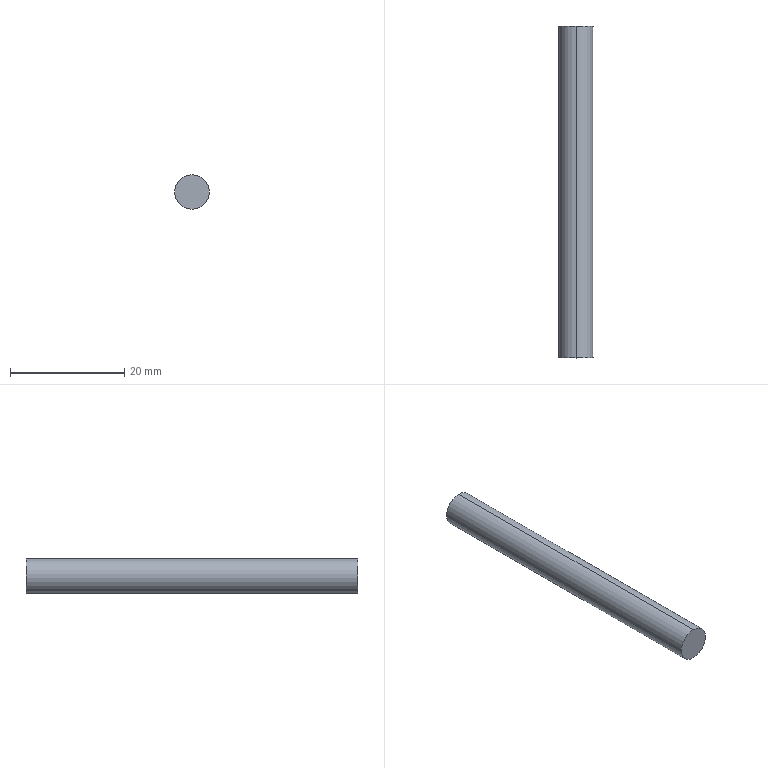Part | SolidWorks | features Extrusion 1 | 1 solid | 4 faces | box 6 x 58 x 6 mm | volume 1640 mm3 | cylinder 2 | plane 2 | commonest cylinder face diameters 6 x2
STEP:
#1=CARTESIAN_POINT('',(0.,58.,3.));
#2=VERTEX_POINT('',#1);
#3=CARTESIAN_POINT('',(0.,58.,-3.));
#4=VERTEX_POINT('',#3);
#5=CARTESIAN_POINT('',(0.,58.,0.));
#6=DIRECTION('',(0.,1.,0.));
#7=DIRECTION('',(0.,0.,1.));
#8=AXIS2_PLACEMENT_3D('',#5,#6,#7);
#9=CIRCLE('',#8,3.);
#10=EDGE_CURVE('',#2,#4,#9,.T.);
#11=ORIENTED_EDGE('',*,*,#10,.F.);
#12=CARTESIAN_POINT('',(0.,0.,3.));
#13=VERTEX_POINT('',#12);
#14=CARTESIAN_POINT('',(0.,58.,3.));
#15=DIRECTION('',(0.,-1.,0.));
#16=VECTOR('',#15,1000.);
#17=LINE('',#14,#16);
#18=EDGE_CURVE('',#2,#13,#17,.T.);
#19=ORIENTED_EDGE('',*,*,#18,.T.);
#20=CARTESIAN_POINT('',(0.,0.,-3.));
#21=VERTEX_POINT('',#20);
#22=CARTESIAN_POINT('',(0.,0.,0.));
#23=DIRECTION('',(0.,1.,0.));
#24=DIRECTION('',(0.,0.,1.));
#25=AXIS2_PLACEMENT_3D('',#22,#23,#24);
#26=CIRCLE('',#25,3.);
#27=EDGE_CURVE('',#13,#21,#26,.T.);
#28=ORIENTED_EDGE('',*,*,#27,.T.);
#29=CARTESIAN_POINT('',(0.,58.,-3.));
#30=DIRECTION('',(0.,-1.,0.));
#31=VECTOR('',#30,1000.);
#32=LINE('',#29,#31);
#33=EDGE_CURVE('',#4,#21,#32,.T.);
#34=ORIENTED_EDGE('',*,*,#33,.F.);
#35=EDGE_LOOP('',(#11,#19,#28,#34));
#36=FACE_OUTER_BOUND('',#35,.T.);
#37=CARTESIAN_POINT('',(0.,58.,0.));
#38=DIRECTION('',(0.,-1.,0.));
#39=DIRECTION('',(0.,0.,-1.));
#40=AXIS2_PLACEMENT_3D('',#37,#38,#39);
#41=CYLINDRICAL_SURFACE('',#40,3.);
#42=ADVANCED_FACE('',(#36),#41,.T.);
#43=ORIENTED_EDGE('',*,*,#18,.F.);
#44=CARTESIAN_POINT('',(0.,58.,0.));
#45=DIRECTION('',(0.,1.,0.));
#46=DIRECTION('',(0.,0.,1.));
#47=AXIS2_PLACEMENT_3D('',#44,#45,#46);
#48=CIRCLE('',#47,3.);
#49=EDGE_CURVE('',#4,#2,#48,.T.);
#50=ORIENTED_EDGE('',*,*,#49,.F.);
#51=ORIENTED_EDGE('',*,*,#33,.T.);
#52=CARTESIAN_POINT('',(0.,0.,0.));
#53=DIRECTION('',(0.,1.,0.));
#54=DIRECTION('',(0.,0.,1.));
#55=AXIS2_PLACEMENT_3D('',#52,#53,#54);
#56=CIRCLE('',#55,3.);
#57=EDGE_CURVE('',#21,#13,#56,.T.);
#58=ORIENTED_EDGE('',*,*,#57,.T.);
#59=EDGE_LOOP('',(#43,#50,#51,#58));
#60=FACE_OUTER_BOUND('',#59,.T.);
#61=CARTESIAN_POINT('',(0.,58.,0.));
#62=DIRECTION('',(0.,-1.,0.));
#63=DIRECTION('',(0.,0.,-1.));
#64=AXIS2_PLACEMENT_3D('',#61,#62,#63);
#65=CYLINDRICAL_SURFACE('',#64,3.);
#66=ADVANCED_FACE('',(#60),#65,.T.);
#67=ORIENTED_EDGE('',*,*,#49,.T.);
#68=ORIENTED_EDGE('',*,*,#10,.T.);
#69=EDGE_LOOP('',(#67,#68));
#70=FACE_OUTER_BOUND('',#69,.T.);
#71=CARTESIAN_POINT('',(0.,58.,0.));
#72=DIRECTION('',(0.,1.,0.));
#73=DIRECTION('',(0.,0.,1.));
#74=AXIS2_PLACEMENT_3D('',#71,#72,#73);
#75=PLANE('',#74);
#76=ADVANCED_FACE('',(#70),#75,.T.);
#77=ORIENTED_EDGE('',*,*,#57,.F.);
#78=ORIENTED_EDGE('',*,*,#27,.F.);
#79=EDGE_LOOP('',(#77,#78));
#80=FACE_OUTER_BOUND('',#79,.T.);
#81=CARTESIAN_POINT('',(0.,0.,0.));
#82=DIRECTION('',(0.,1.,0.));
#83=DIRECTION('',(0.,0.,1.));
#84=AXIS2_PLACEMENT_3D('',#81,#82,#83);
#85=PLANE('',#84);
#86=ADVANCED_FACE('',(#80),#85,.F.);
#87=CLOSED_SHELL('',(#42,#66,#76,#86));
#88=MANIFOLD_SOLID_BREP('',#87);
#89=CARTESIAN_POINT('',(0.,0.,0.));
#90=DIRECTION('',(0.,0.,1.));
#91=DIRECTION('',(1.,0.,0.));
#92=AXIS2_PLACEMENT_3D('',#89,#90,#91);
#93=(LENGTH_UNIT()NAMED_UNIT(*)SI_UNIT(.MILLI.,.METRE.));
#94=UNCERTAINTY_MEASURE_WITH_UNIT(LENGTH_MEASURE(0.00001),#93,'','');
#95=(NAMED_UNIT(*)PLANE_ANGLE_UNIT()SI_UNIT($,.RADIAN.));
#96=(NAMED_UNIT(*)SI_UNIT($,.STERADIAN.)SOLID_ANGLE_UNIT());
#97=(GEOMETRIC_REPRESENTATION_CONTEXT(3)GLOBAL_UNCERTAINTY_ASSIGNED_CONTEXT((#94))GLOBAL_UNIT_ASSIGNED_CONTEXT((#93,#95,#96))REPRESENTATION_CONTEXT('',''));
#98=ADVANCED_BREP_SHAPE_REPRESENTATION('',(#88,#92),#97);